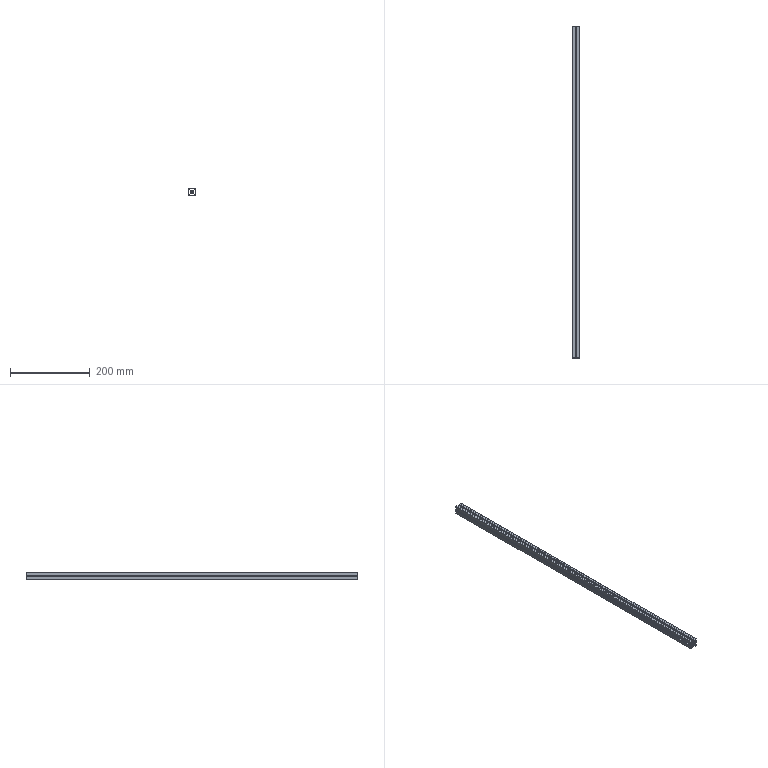Part | STEP file | 20 aluminium profile longitudinal 1 | 1 solid | 64 faces | box 20 x 830 x 20 mm | volume 147557 mm3 | plane 54 | cylinder 10 | commonest cylinder face diameters 3.3 x10